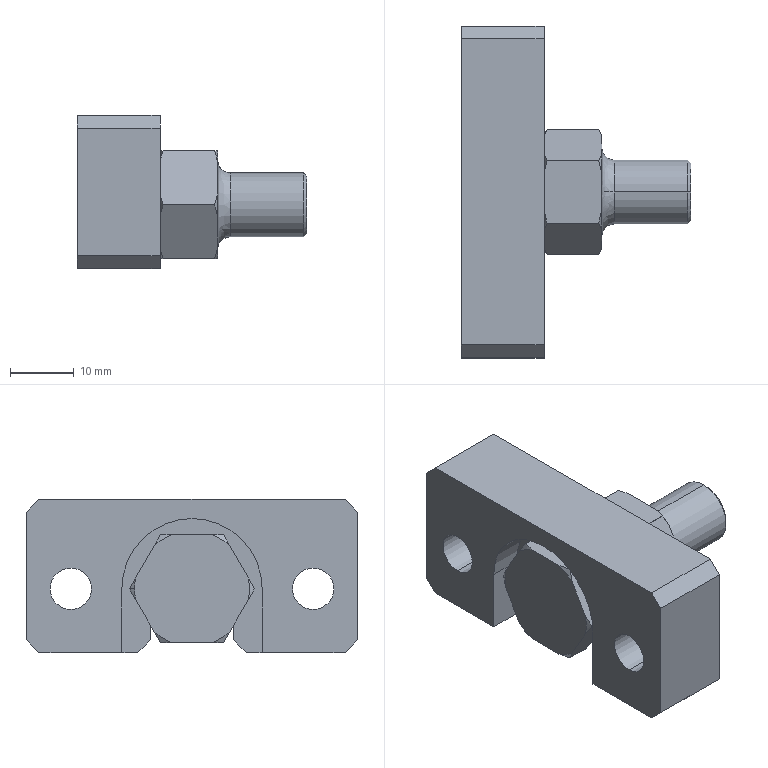Part | SolidWorks | features BaseBody 2, Chamfer 1, ICE 1 | 2 solids | 98 faces | box 36 x 52 x 24 mm | volume 16208 mm3 | plane 37 | cone 28 | cylinder 27 | spline 6 | commonest cylinder face diameters 19.6 x12 6.5 x4 11 x4 10 x2 12 x2 22 x2